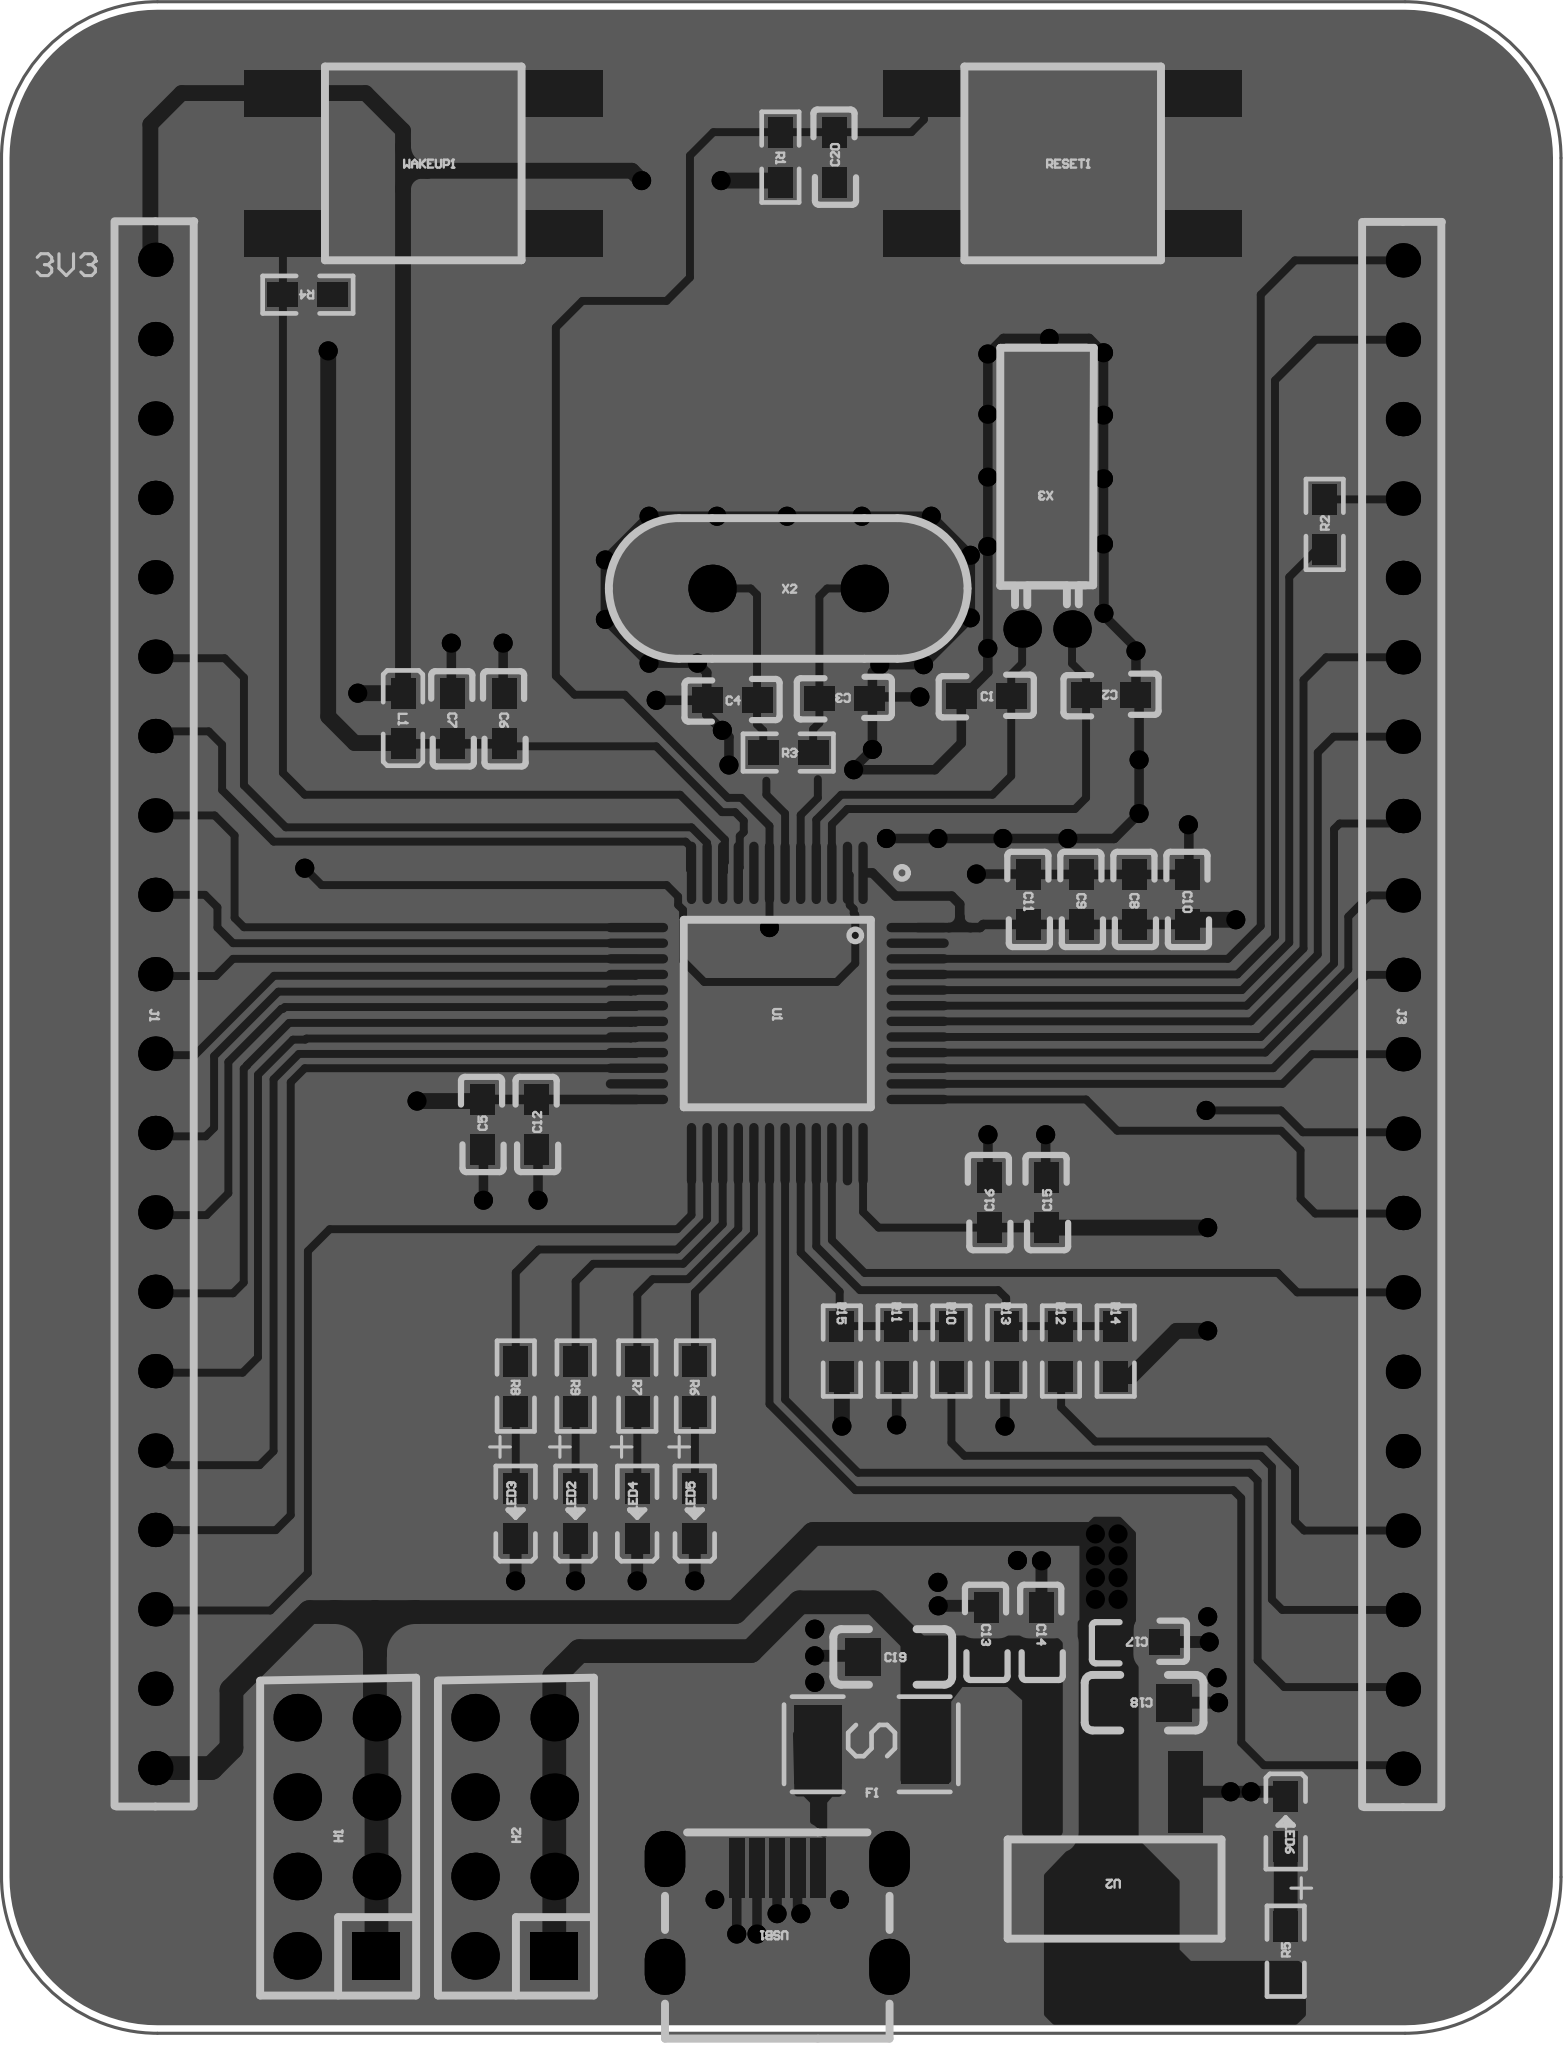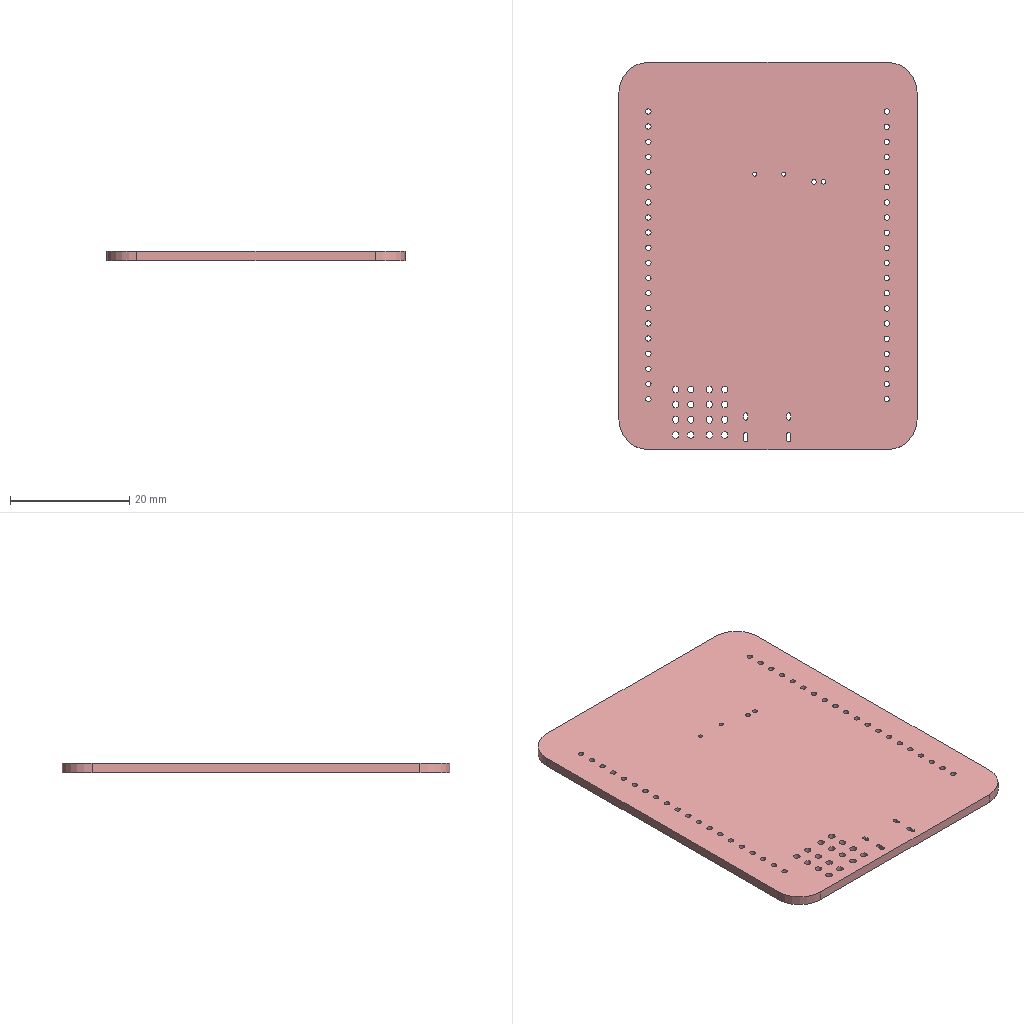Circuit board layout | Altium Designer | box 50 x 65 x 1.6 mm
Layer stack:
# Altium Designer layer stack of  (unit mm; dielectric type: 0 none, 1 core, 2 prepreg, 3 surface material)
index,name,kind,layer,copper_thickness_mm,dielectric_type,dielectric_thickness_mm,dielectric_material,dielectric_constant
0,Top Paste Mask Layer,other,,,,,,
1,Top Silkscreen Layer,other,,,,,,
2,Top Solder Mask Layer,dielectric,,,3,0.01,,3.3
3,Top Layer,copper,Top Layer,0.035,,,,
4,Dielectric1,dielectric,,,3,1.51,FR4,4.5
5,Bottom Layer,copper,Bottom Layer,0.035,,,,
6,Bottom Solder Mask Layer,dielectric,,,3,0.01,,3.3
7,Bottom Silkscreen Layer,other,,,,,,
8,Bottom Paste Mask Layer,other,,,,,,
# drill layer pairs: low layer,high layer
drill_pair,Top Layer,Bottom Layer
Part placement:
Designator,Comment,Layer,Footprint,Center-X(mm),Center-Y(mm),Rotation
C1,20pF,TopLayer,C0603,109.65,122.308,0
C2,20pF,TopLayer,C0603,113.65,122.342,180
C3,20pF,TopLayer,C0603,105.1,122.242,180
C4,20pF,TopLayer,C0603,101.5,122.172,0
C5,1uF,TopLayer,C0603,93.492,108.6,90
C6,10nF,TopLayer,C0603,94.198,121.578,270
C7,1uF,TopLayer,C0603,92.537,121.578,270
C8,1uF,TopLayer,C0603,114.408,115.8,270
C9,10nF,TopLayer,C0603,112.708,115.8,270
C10,1uF,TopLayer,C0603,116.108,115.8,270
C11,10nF,TopLayer,C0603,111.008,115.8,270
C12,10nF,TopLayer,C0603,95.242,108.6,90
C13,1uF,TopLayer,C0603,109.65,92.35,270
C14,10nF,TopLayer,C0603,111.42,92.35,270
C15,1uF,TopLayer,C0603,111.592,106.1,90
C16,10nF,TopLayer,C0603,109.742,106.1,90
C17,100nf,TopLayer,C0603,114.56,92.042,180
C18,10uf,TopLayer,C0805,114.71,90.1,180
C19,22uF,TopLayer,C0805,106.652,91.564,0
C20,100nF,TopLayer,C0603,104.792,139.55,90
F1,,TopLayer,F1210,105.96,88.77,0
H1,,TopLayer,HDR-TH_8P-P2.54-V-M-R2-C4-S2.54,88.83,85.81,90
H2,,TopLayer,HDR-TH_8P-P2.54-V-M-R2-C4-S2.54,94.53,85.81,90
J1,,TopLayer,HDR-TH_20PIN-V-MALE-PITCH2.54,83.01,112.138,270
J3,,TopLayer,HDR-TH_20PIN-V-MALE-PITCH2.54,123.01,112.118,270
L1,3.3uH,TopLayer,L0603,90.95,121.603,270
LED2,,TopLayer,LED0603,96.48,96.15,90
LED3,,TopLayer,LED0603,94.56,96.15,90
LED4,,TopLayer,LED0603,98.457,96.15,90
LED5,,TopLayer,LED0603,100.305,96.15,90
LED6,,TopLayer,LED0603,119.25,86.3,270
R1,10K,TopLayer,R0603,103.05,139.55,270
R2,10K,TopLayer,R0603,120.5,127.8,90
R3,1M,TopLayer,R0603,103.3,120.5,0
R4,10K,TopLayer,R0603,87.9,135.15,180
R5,1K,TopLayer,R0603,119.25,82.15,90
R6,1K,TopLayer,R0603,100.31,100.231,270
R7,1K,TopLayer,R0603,98.462,100.231,270
R8,1K,TopLayer,R0603,94.565,100.231,270
R9,1K,TopLayer,R0603,96.485,100.231,270
R10,0R,TopLayer,R0603,108.533,101.35,270
R11,NC/22R,TopLayer,R0603,106.777,101.35,270
R12,0R,TopLayer,R0603,112.044,101.35,270
R13,NC/22R,TopLayer,R0603,110.288,101.35,270
R14,NC/1.5K,TopLayer,R0603,113.8,101.35,270
R15,NC/1.5K,TopLayer,R0603,105.021,101.35,270
RESET1,,TopLayer,SW-SMD-T6X6-9.5X5.8,112.1,139.35,0
U1,,TopLayer,TQFP-48_L7.0-W7.0-P0.50-LS9.0-BL,102.95,112.15,180
U2,,TopLayer,SOT-223,113.76,84.25,180
USB1,,TopLayer,U-F-M5DD-Y-1,102.95,83.375,180
WAKEUP1,,TopLayer,SW-SMD-T6X6-9.5X5.8,91.6,139.35,0
X2,8MHz,TopLayer,OSC-49S-1,103.3,125.75,0
X3,32.768kHz,TopLayer,DT-38_BD3.1-P0.80,111.6,124.45,180
Pad and via stacks:
# Altium Designer via and pad stacks of  (unit mm). Each distinct definition once, with the count of objects using it.
# via: kind,start_layer,end_layer,hole_mm,diameter_mm,mode(0 simple;1 top-mid-bottom;2 full stack),diameter_per_layer,count,example_net
# pad: kind,layer,hole_mm,hole_type(0 round;1 square;2 slot),plating,top_size,top_shape(1 round;2 rect;3 octagon;9 rounded rect),mid_size,bottom_size,mode,footprint,size_per_layer,count,example
pad,Top Layer,0,0,plated,0.965x0.8,2,0.965x0.8,0.965x0.8,0,C0603,,36,C1.1
pad,Top Layer,0,0,plated,1.14x1.2,2,1.14x1.2,1.14x1.2,0,C0805,,4,C18.1
pad,Top Layer,0,0,plated,1.52x2.5,2,1.52x2.5,1.52x2.5,0,F1210,,2,F1.1
pad,Top Layer,0,0,plated,0.965x0.8,2,0.965x0.8,0.965x0.8,0,L0603,,2,L1.1
pad,Top Layer,0,0,plated,0.965x0.8,2,0.965x0.8,0.965x0.8,0,LED0603,,10,LED2.1
pad,Top Layer,0,0,plated,0.965x0.8,2,0.965x0.8,0.965x0.8,0,R0603,,30,R1.1
pad,Top Layer,0,0,plated,1.5x2.5,2,1.5x2.5,1.5x2.5,0,SW-SMD-T6X6-9.5X5.8,,8,RESET1.1
pad,Top Layer,0,0,plated,2x0.3,1,2x0.3,2x0.3,0,TQFP-48_L7.0-W7.0-P0.50-LS9.0-BL,,48,U1.1
pad,Top Layer,0,0,plated,1.1x2.6,2,1.1x2.6,1.1x2.6,0,SOT-223,,3,U2.1
pad,Top Layer,0,0,plated,3.6x2.4,2,3.6x2.4,3.6x2.4,0,SOT-223,,1,U2.4
pad,Top Layer,0,0,plated,0.5x1.9,2,0.5x1.9,0.5x1.9,0,U-F-M5DD-Y-1,,5,USB1.1
pad,Multi-Layer,1.1,0,plated,1.524x1.524,2,1.524x1.524,1.524x1.524,0,HDR-TH_8P-P2.54-V-M-R2-C4-S2.54,,2,H1.1
pad,Multi-Layer,1.1,0,plated,1.524x1.524,1,1.524x1.524,1.524x1.524,0,HDR-TH_8P-P2.54-V-M-R2-C4-S2.54,,14,H1.2
pad,Multi-Layer,0.9144,0,plated,1.1x1.1,1,1.1x1.1,1.1x1.1,0,HDR-TH_20PIN-V-MALE-PITCH2.54,,40,J1.1
pad,Multi-Layer,0.65,2,plated,1.3x1.8,1,1.3x1.8,1.3x1.8,0,U-F-M5DD-Y-1,,2,USB1.6
pad,Multi-Layer,0.7,2,plated,1.3x1.8,1,1.3x1.8,1.3x1.8,0,U-F-M5DD-Y-1,,2,USB1.8
pad,Multi-Layer,0.7,0,plated,1.524x1.524,1,1.524x1.524,1.524x1.524,0,OSC-49S-1,,2,X2.1
pad,Multi-Layer,0.8,0,plated,1.2x1.2,1,1.2x1.2,1.2x1.2,0,DT-38_BD3.1-P0.80,,2,X3.1
via,Top Layer,Bottom Layer,0.3048,0.61,0,,88,GND
via,Top Layer,Bottom Layer,0.5994,0.6,0,,2,
Copper pours:
name,layer,net,type(0 solid;1 hatched;2 none)
Top Layer-$1N3542,Top Layer,$1N3542,0
Top Layer-VIN_5V,Top Layer,VIN_5V,0
Top Layer-VIN_5V 1,Top Layer,VIN_5V,0
Top Layer-VCC_3V3,Top Layer,VCC_3V3,0
Top Layer-VCC_3V3 1,Top Layer,VCC_3V3,0
Bottom Layer-VCC_3V3,Bottom Layer,VCC_3V3,0
Bottom Layer-VCC_3V3 1,Bottom Layer,VCC_3V3,0
Bottom Layer-GND,Bottom Layer,GND,0
Design rules, without the lines most boards share:
# Altium Designer design rules of  (exported by Altium Designer, unit mm)
# columns: name | kind | enabled | priority | scope1 | scope2 | descriptor | typed fields (field=value)
power | 2 | enabled | 2 | (InNet('GND') OR InNet('VCC_3V3') OR InNet('VDDA') OR InNet('VIN_5V')) | All | Width Constraint (Min=10mil) (Max=100mil) (Preferred=30mil) ((InNet('GND') OR InNet('VCC_3V3') OR InNet('VDDA') OR InNet('VIN_5V'))) |
copperThickness1oz_2 | 2 | enabled | 3 | All | All | Width Constraint (Min=5mil) (Max=100mil) (Preferred=10mil) (All) |
copperRegion | 20 | enabled | 1 | All | All | Polygon Connect Rule(Direct Connect )(Conductor Width=10mil) (Relief Angle=90 Angle) (Entries=4) (Air Gap Width=10mil) (All),(All) | connect_style(0=relief,1=direct,2=none)=1 relief_conductor_width=0.254 relief_entries=4